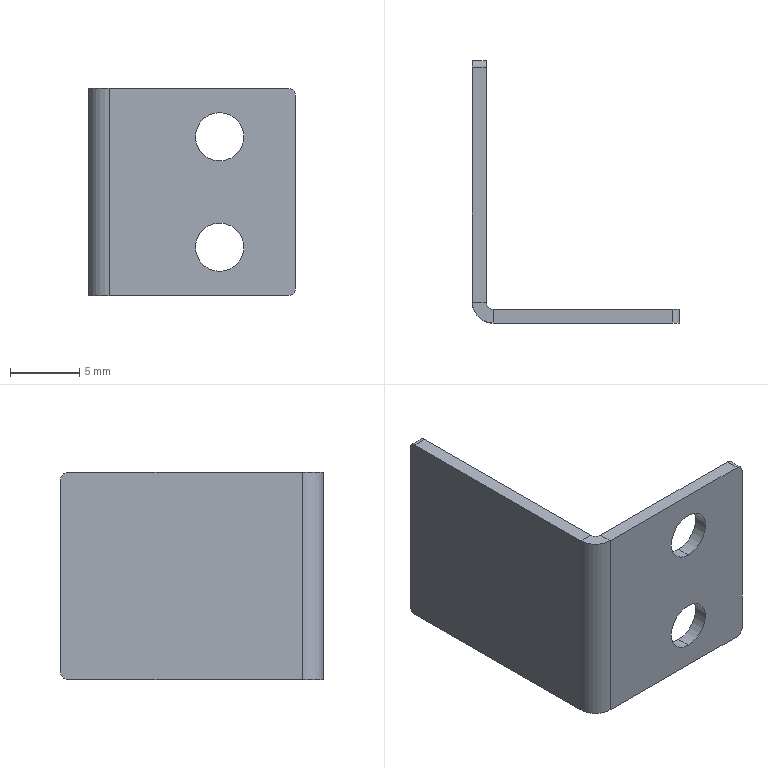Part | STEP file | 1 solid | 22 faces | box 15 x 19 x 15 mm | volume 469.105 mm3 | plane 12 | cylinder 10 | commonest cylinder face diameters 1 x5 3.5 x4 3 x1